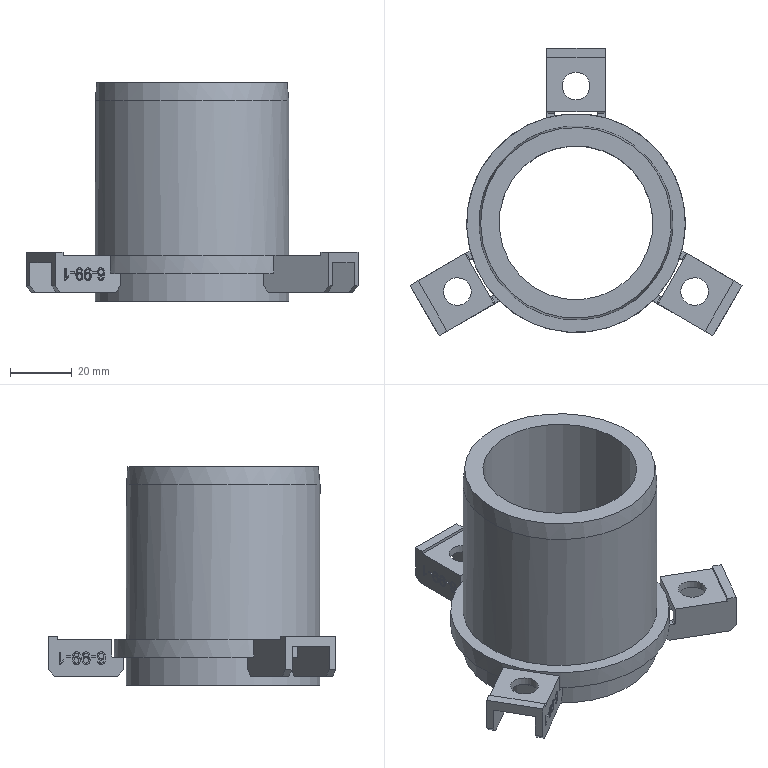Part | STEP file | lll_id3034_x_t | 1 solid | 301 faces | box 107.83 x 93.384 x 71 mm | volume 91487 mm3 | plane 198 | other 88 | cylinder 13 | torus 1 | cone 1 | commonest cylinder face diameters 1 x6 9 x3 50 x1 62.98 x1 63 x1 71 x1